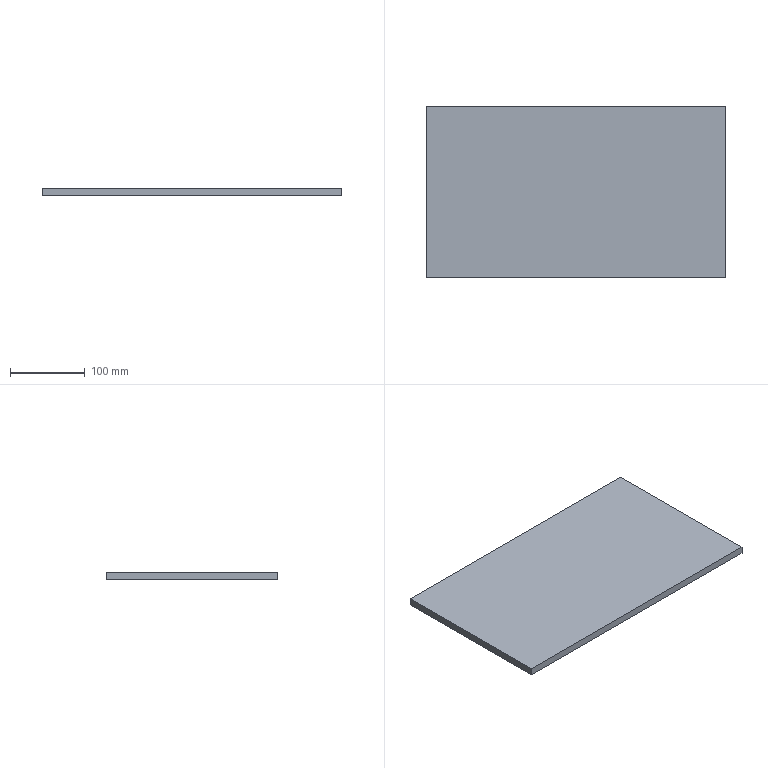Part | SolidWorks | features Extrusion 1 | 1 solid | 6 faces | box 400 x 230 x 10 mm | volume 920000 mm3 | plane 6
STEP:
#1=CARTESIAN_POINT('',(-200.,115.,0.));
#2=VERTEX_POINT('',#1);
#3=CARTESIAN_POINT('',(-200.,-115.,0.));
#4=VERTEX_POINT('',#3);
#5=CARTESIAN_POINT('',(-200.,-115.,0.));
#6=DIRECTION('',(0.,-1.,0.));
#7=VECTOR('',#6,1000.);
#8=LINE('',#5,#7);
#9=EDGE_CURVE('',#2,#4,#8,.T.);
#10=ORIENTED_EDGE('',*,*,#9,.T.);
#11=CARTESIAN_POINT('',(-200.,-115.,10.));
#12=VERTEX_POINT('',#11);
#13=CARTESIAN_POINT('',(-200.,-115.,10.));
#14=DIRECTION('',(0.,0.,-1.));
#15=VECTOR('',#14,1000.);
#16=LINE('',#13,#15);
#17=EDGE_CURVE('',#12,#4,#16,.T.);
#18=ORIENTED_EDGE('',*,*,#17,.F.);
#19=CARTESIAN_POINT('',(-200.,115.,10.));
#20=VERTEX_POINT('',#19);
#21=CARTESIAN_POINT('',(-200.,-115.,10.));
#22=DIRECTION('',(0.,-1.,0.));
#23=VECTOR('',#22,1000.);
#24=LINE('',#21,#23);
#25=EDGE_CURVE('',#20,#12,#24,.T.);
#26=ORIENTED_EDGE('',*,*,#25,.F.);
#27=CARTESIAN_POINT('',(-200.,115.,10.));
#28=DIRECTION('',(0.,0.,-1.));
#29=VECTOR('',#28,1000.);
#30=LINE('',#27,#29);
#31=EDGE_CURVE('',#20,#2,#30,.T.);
#32=ORIENTED_EDGE('',*,*,#31,.T.);
#33=EDGE_LOOP('',(#10,#18,#26,#32));
#34=FACE_OUTER_BOUND('',#33,.T.);
#35=CARTESIAN_POINT('',(-200.,-115.,10.));
#36=DIRECTION('',(1.,0.,0.));
#37=DIRECTION('',(0.,0.,-1.));
#38=AXIS2_PLACEMENT_3D('',#35,#36,#37);
#39=PLANE('',#38);
#40=ADVANCED_FACE('',(#34),#39,.F.);
#41=CARTESIAN_POINT('',(200.,-115.,0.));
#42=VERTEX_POINT('',#41);
#43=CARTESIAN_POINT('',(200.,-115.,0.));
#44=DIRECTION('',(1.,0.,0.));
#45=VECTOR('',#44,1000.);
#46=LINE('',#43,#45);
#47=EDGE_CURVE('',#4,#42,#46,.T.);
#48=ORIENTED_EDGE('',*,*,#47,.T.);
#49=CARTESIAN_POINT('',(200.,-115.,10.));
#50=VERTEX_POINT('',#49);
#51=CARTESIAN_POINT('',(200.,-115.,10.));
#52=DIRECTION('',(0.,0.,-1.));
#53=VECTOR('',#52,1000.);
#54=LINE('',#51,#53);
#55=EDGE_CURVE('',#50,#42,#54,.T.);
#56=ORIENTED_EDGE('',*,*,#55,.F.);
#57=CARTESIAN_POINT('',(200.,-115.,10.));
#58=DIRECTION('',(1.,0.,0.));
#59=VECTOR('',#58,1000.);
#60=LINE('',#57,#59);
#61=EDGE_CURVE('',#12,#50,#60,.T.);
#62=ORIENTED_EDGE('',*,*,#61,.F.);
#63=ORIENTED_EDGE('',*,*,#17,.T.);
#64=EDGE_LOOP('',(#48,#56,#62,#63));
#65=FACE_OUTER_BOUND('',#64,.T.);
#66=CARTESIAN_POINT('',(200.,-115.,10.));
#67=DIRECTION('',(0.,1.,0.));
#68=DIRECTION('',(-1.,0.,0.));
#69=AXIS2_PLACEMENT_3D('',#66,#67,#68);
#70=PLANE('',#69);
#71=ADVANCED_FACE('',(#65),#70,.F.);
#72=CARTESIAN_POINT('',(200.,115.,0.));
#73=VERTEX_POINT('',#72);
#74=CARTESIAN_POINT('',(200.,-115.,0.));
#75=DIRECTION('',(0.,1.,0.));
#76=VECTOR('',#75,1000.);
#77=LINE('',#74,#76);
#78=EDGE_CURVE('',#42,#73,#77,.T.);
#79=ORIENTED_EDGE('',*,*,#78,.T.);
#80=CARTESIAN_POINT('',(200.,115.,10.));
#81=VERTEX_POINT('',#80);
#82=CARTESIAN_POINT('',(200.,115.,10.));
#83=DIRECTION('',(0.,0.,-1.));
#84=VECTOR('',#83,1000.);
#85=LINE('',#82,#84);
#86=EDGE_CURVE('',#81,#73,#85,.T.);
#87=ORIENTED_EDGE('',*,*,#86,.F.);
#88=CARTESIAN_POINT('',(200.,-115.,10.));
#89=DIRECTION('',(0.,1.,0.));
#90=VECTOR('',#89,1000.);
#91=LINE('',#88,#90);
#92=EDGE_CURVE('',#50,#81,#91,.T.);
#93=ORIENTED_EDGE('',*,*,#92,.F.);
#94=ORIENTED_EDGE('',*,*,#55,.T.);
#95=EDGE_LOOP('',(#79,#87,#93,#94));
#96=FACE_OUTER_BOUND('',#95,.T.);
#97=CARTESIAN_POINT('',(200.,-115.,10.));
#98=DIRECTION('',(-1.,0.,0.));
#99=DIRECTION('',(0.,0.,1.));
#100=AXIS2_PLACEMENT_3D('',#97,#98,#99);
#101=PLANE('',#100);
#102=ADVANCED_FACE('',(#96),#101,.F.);
#103=CARTESIAN_POINT('',(200.,115.,0.));
#104=DIRECTION('',(-1.,0.,0.));
#105=VECTOR('',#104,1000.);
#106=LINE('',#103,#105);
#107=EDGE_CURVE('',#73,#2,#106,.T.);
#108=ORIENTED_EDGE('',*,*,#107,.T.);
#109=ORIENTED_EDGE('',*,*,#31,.F.);
#110=CARTESIAN_POINT('',(200.,115.,10.));
#111=DIRECTION('',(-1.,0.,0.));
#112=VECTOR('',#111,1000.);
#113=LINE('',#110,#112);
#114=EDGE_CURVE('',#81,#20,#113,.T.);
#115=ORIENTED_EDGE('',*,*,#114,.F.);
#116=ORIENTED_EDGE('',*,*,#86,.T.);
#117=EDGE_LOOP('',(#108,#109,#115,#116));
#118=FACE_OUTER_BOUND('',#117,.T.);
#119=CARTESIAN_POINT('',(200.,115.,10.));
#120=DIRECTION('',(0.,-1.,0.));
#121=DIRECTION('',(1.,0.,0.));
#122=AXIS2_PLACEMENT_3D('',#119,#120,#121);
#123=PLANE('',#122);
#124=ADVANCED_FACE('',(#118),#123,.F.);
#125=ORIENTED_EDGE('',*,*,#25,.T.);
#126=ORIENTED_EDGE('',*,*,#61,.T.);
#127=ORIENTED_EDGE('',*,*,#92,.T.);
#128=ORIENTED_EDGE('',*,*,#114,.T.);
#129=EDGE_LOOP('',(#125,#126,#127,#128));
#130=FACE_OUTER_BOUND('',#129,.T.);
#131=CARTESIAN_POINT('',(0.,0.,10.));
#132=DIRECTION('',(0.,0.,1.));
#133=DIRECTION('',(1.,0.,0.));
#134=AXIS2_PLACEMENT_3D('',#131,#132,#133);
#135=PLANE('',#134);
#136=ADVANCED_FACE('',(#130),#135,.T.);
#137=ORIENTED_EDGE('',*,*,#9,.F.);
#138=ORIENTED_EDGE('',*,*,#107,.F.);
#139=ORIENTED_EDGE('',*,*,#78,.F.);
#140=ORIENTED_EDGE('',*,*,#47,.F.);
#141=EDGE_LOOP('',(#137,#138,#139,#140));
#142=FACE_OUTER_BOUND('',#141,.T.);
#143=CARTESIAN_POINT('',(0.,0.,0.));
#144=DIRECTION('',(0.,0.,1.));
#145=DIRECTION('',(1.,0.,0.));
#146=AXIS2_PLACEMENT_3D('',#143,#144,#145);
#147=PLANE('',#146);
#148=ADVANCED_FACE('',(#142),#147,.F.);
#149=CLOSED_SHELL('',(#40,#71,#102,#124,#136,#148));
#150=MANIFOLD_SOLID_BREP('',#149);
#151=CARTESIAN_POINT('',(0.,0.,0.));
#152=DIRECTION('',(0.,0.,1.));
#153=DIRECTION('',(1.,0.,0.));
#154=AXIS2_PLACEMENT_3D('',#151,#152,#153);
#155=(LENGTH_UNIT()NAMED_UNIT(*)SI_UNIT(.MILLI.,.METRE.));
#156=UNCERTAINTY_MEASURE_WITH_UNIT(LENGTH_MEASURE(0.00001),#155,'','');
#157=(NAMED_UNIT(*)PLANE_ANGLE_UNIT()SI_UNIT($,.RADIAN.));
#158=(NAMED_UNIT(*)SI_UNIT($,.STERADIAN.)SOLID_ANGLE_UNIT());
#159=(GEOMETRIC_REPRESENTATION_CONTEXT(3)GLOBAL_UNCERTAINTY_ASSIGNED_CONTEXT((#156))GLOBAL_UNIT_ASSIGNED_CONTEXT((#155,#157,#158))REPRESENTATION_CONTEXT('',''));
#160=ADVANCED_BREP_SHAPE_REPRESENTATION('',(#150,#154),#159);